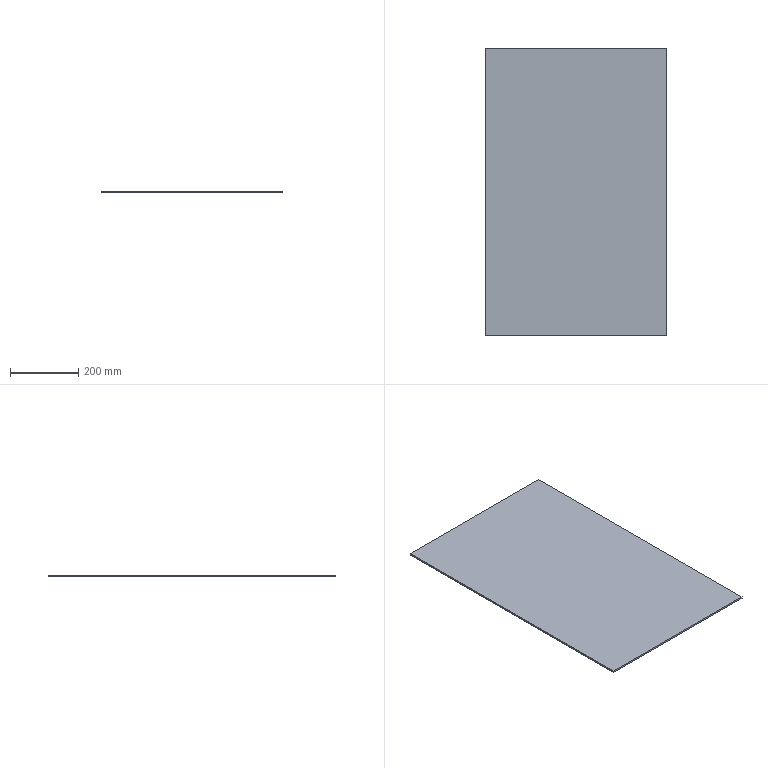Part | SolidWorks | features Extrusion 1, HoleWzd 1 | 1 solid | 6 faces | box 532 x 842 x 5 mm | volume 2239720 mm3 | plane 6
STEP:
#1=CARTESIAN_POINT('',(266.,-421.,0.));
#2=VERTEX_POINT('',#1);
#3=CARTESIAN_POINT('',(266.,421.,0.));
#4=VERTEX_POINT('',#3);
#5=CARTESIAN_POINT('',(266.,421.,0.));
#6=DIRECTION('',(0.,1.,0.));
#7=VECTOR('',#6,1000.);
#8=LINE('',#5,#7);
#9=EDGE_CURVE('',#2,#4,#8,.T.);
#10=ORIENTED_EDGE('',*,*,#9,.T.);
#11=CARTESIAN_POINT('',(266.,421.,5.));
#12=VERTEX_POINT('',#11);
#13=CARTESIAN_POINT('',(266.,421.,5.));
#14=DIRECTION('',(0.,0.,-1.));
#15=VECTOR('',#14,1000.);
#16=LINE('',#13,#15);
#17=EDGE_CURVE('',#12,#4,#16,.T.);
#18=ORIENTED_EDGE('',*,*,#17,.F.);
#19=CARTESIAN_POINT('',(266.,-421.,5.));
#20=VERTEX_POINT('',#19);
#21=CARTESIAN_POINT('',(266.,421.,5.));
#22=DIRECTION('',(0.,1.,0.));
#23=VECTOR('',#22,1000.);
#24=LINE('',#21,#23);
#25=EDGE_CURVE('',#20,#12,#24,.T.);
#26=ORIENTED_EDGE('',*,*,#25,.F.);
#27=CARTESIAN_POINT('',(266.,-421.,5.));
#28=DIRECTION('',(0.,0.,-1.));
#29=VECTOR('',#28,1000.);
#30=LINE('',#27,#29);
#31=EDGE_CURVE('',#20,#2,#30,.T.);
#32=ORIENTED_EDGE('',*,*,#31,.T.);
#33=EDGE_LOOP('',(#10,#18,#26,#32));
#34=FACE_OUTER_BOUND('',#33,.T.);
#35=CARTESIAN_POINT('',(266.,421.,5.));
#36=DIRECTION('',(-1.,0.,0.));
#37=DIRECTION('',(0.,-1.,0.));
#38=AXIS2_PLACEMENT_3D('',#35,#36,#37);
#39=PLANE('',#38);
#40=ADVANCED_FACE('',(#34),#39,.F.);
#41=CARTESIAN_POINT('',(-266.,421.,0.));
#42=VERTEX_POINT('',#41);
#43=CARTESIAN_POINT('',(-266.,421.,0.));
#44=DIRECTION('',(-1.,0.,0.));
#45=VECTOR('',#44,1000.);
#46=LINE('',#43,#45);
#47=EDGE_CURVE('',#4,#42,#46,.T.);
#48=ORIENTED_EDGE('',*,*,#47,.T.);
#49=CARTESIAN_POINT('',(-266.,421.,5.));
#50=VERTEX_POINT('',#49);
#51=CARTESIAN_POINT('',(-266.,421.,5.));
#52=DIRECTION('',(0.,0.,-1.));
#53=VECTOR('',#52,1000.);
#54=LINE('',#51,#53);
#55=EDGE_CURVE('',#50,#42,#54,.T.);
#56=ORIENTED_EDGE('',*,*,#55,.F.);
#57=CARTESIAN_POINT('',(-266.,421.,5.));
#58=DIRECTION('',(-1.,0.,0.));
#59=VECTOR('',#58,1000.);
#60=LINE('',#57,#59);
#61=EDGE_CURVE('',#12,#50,#60,.T.);
#62=ORIENTED_EDGE('',*,*,#61,.F.);
#63=ORIENTED_EDGE('',*,*,#17,.T.);
#64=EDGE_LOOP('',(#48,#56,#62,#63));
#65=FACE_OUTER_BOUND('',#64,.T.);
#66=CARTESIAN_POINT('',(-266.,421.,5.));
#67=DIRECTION('',(0.,-1.,0.));
#68=DIRECTION('',(0.,0.,-1.));
#69=AXIS2_PLACEMENT_3D('',#66,#67,#68);
#70=PLANE('',#69);
#71=ADVANCED_FACE('',(#65),#70,.F.);
#72=CARTESIAN_POINT('',(-266.,-421.,0.));
#73=VERTEX_POINT('',#72);
#74=CARTESIAN_POINT('',(-266.,421.,0.));
#75=DIRECTION('',(0.,-1.,0.));
#76=VECTOR('',#75,1000.);
#77=LINE('',#74,#76);
#78=EDGE_CURVE('',#42,#73,#77,.T.);
#79=ORIENTED_EDGE('',*,*,#78,.T.);
#80=CARTESIAN_POINT('',(-266.,-421.,5.));
#81=VERTEX_POINT('',#80);
#82=CARTESIAN_POINT('',(-266.,-421.,5.));
#83=DIRECTION('',(0.,0.,-1.));
#84=VECTOR('',#83,1000.);
#85=LINE('',#82,#84);
#86=EDGE_CURVE('',#81,#73,#85,.T.);
#87=ORIENTED_EDGE('',*,*,#86,.F.);
#88=CARTESIAN_POINT('',(-266.,421.,5.));
#89=DIRECTION('',(0.,-1.,0.));
#90=VECTOR('',#89,1000.);
#91=LINE('',#88,#90);
#92=EDGE_CURVE('',#50,#81,#91,.T.);
#93=ORIENTED_EDGE('',*,*,#92,.F.);
#94=ORIENTED_EDGE('',*,*,#55,.T.);
#95=EDGE_LOOP('',(#79,#87,#93,#94));
#96=FACE_OUTER_BOUND('',#95,.T.);
#97=CARTESIAN_POINT('',(-266.,421.,5.));
#98=DIRECTION('',(1.,0.,0.));
#99=DIRECTION('',(0.,1.,0.));
#100=AXIS2_PLACEMENT_3D('',#97,#98,#99);
#101=PLANE('',#100);
#102=ADVANCED_FACE('',(#96),#101,.F.);
#103=CARTESIAN_POINT('',(-266.,-421.,0.));
#104=DIRECTION('',(1.,0.,0.));
#105=VECTOR('',#104,1000.);
#106=LINE('',#103,#105);
#107=EDGE_CURVE('',#73,#2,#106,.T.);
#108=ORIENTED_EDGE('',*,*,#107,.T.);
#109=ORIENTED_EDGE('',*,*,#31,.F.);
#110=CARTESIAN_POINT('',(-266.,-421.,5.));
#111=DIRECTION('',(1.,0.,0.));
#112=VECTOR('',#111,1000.);
#113=LINE('',#110,#112);
#114=EDGE_CURVE('',#81,#20,#113,.T.);
#115=ORIENTED_EDGE('',*,*,#114,.F.);
#116=ORIENTED_EDGE('',*,*,#86,.T.);
#117=EDGE_LOOP('',(#108,#109,#115,#116));
#118=FACE_OUTER_BOUND('',#117,.T.);
#119=CARTESIAN_POINT('',(-266.,-421.,5.));
#120=DIRECTION('',(0.,1.,0.));
#121=DIRECTION('',(0.,0.,1.));
#122=AXIS2_PLACEMENT_3D('',#119,#120,#121);
#123=PLANE('',#122);
#124=ADVANCED_FACE('',(#118),#123,.F.);
#125=ORIENTED_EDGE('',*,*,#25,.T.);
#126=ORIENTED_EDGE('',*,*,#61,.T.);
#127=ORIENTED_EDGE('',*,*,#92,.T.);
#128=ORIENTED_EDGE('',*,*,#114,.T.);
#129=EDGE_LOOP('',(#125,#126,#127,#128));
#130=FACE_OUTER_BOUND('',#129,.T.);
#131=CARTESIAN_POINT('',(0.,0.,5.));
#132=DIRECTION('',(0.,0.,1.));
#133=DIRECTION('',(1.,0.,0.));
#134=AXIS2_PLACEMENT_3D('',#131,#132,#133);
#135=PLANE('',#134);
#136=ADVANCED_FACE('',(#130),#135,.T.);
#137=ORIENTED_EDGE('',*,*,#9,.F.);
#138=ORIENTED_EDGE('',*,*,#107,.F.);
#139=ORIENTED_EDGE('',*,*,#78,.F.);
#140=ORIENTED_EDGE('',*,*,#47,.F.);
#141=EDGE_LOOP('',(#137,#138,#139,#140));
#142=FACE_OUTER_BOUND('',#141,.T.);
#143=CARTESIAN_POINT('',(0.,0.,0.));
#144=DIRECTION('',(0.,0.,1.));
#145=DIRECTION('',(1.,0.,0.));
#146=AXIS2_PLACEMENT_3D('',#143,#144,#145);
#147=PLANE('',#146);
#148=ADVANCED_FACE('',(#142),#147,.F.);
#149=CLOSED_SHELL('',(#40,#71,#102,#124,#136,#148));
#150=MANIFOLD_SOLID_BREP('',#149);
#151=CARTESIAN_POINT('',(0.,0.,0.));
#152=DIRECTION('',(0.,0.,1.));
#153=DIRECTION('',(1.,0.,0.));
#154=AXIS2_PLACEMENT_3D('',#151,#152,#153);
#155=(LENGTH_UNIT()NAMED_UNIT(*)SI_UNIT(.MILLI.,.METRE.));
#156=UNCERTAINTY_MEASURE_WITH_UNIT(LENGTH_MEASURE(0.00001),#155,'','');
#157=(NAMED_UNIT(*)PLANE_ANGLE_UNIT()SI_UNIT($,.RADIAN.));
#158=(NAMED_UNIT(*)SI_UNIT($,.STERADIAN.)SOLID_ANGLE_UNIT());
#159=(GEOMETRIC_REPRESENTATION_CONTEXT(3)GLOBAL_UNCERTAINTY_ASSIGNED_CONTEXT((#156))GLOBAL_UNIT_ASSIGNED_CONTEXT((#155,#157,#158))REPRESENTATION_CONTEXT('',''));
#160=ADVANCED_BREP_SHAPE_REPRESENTATION('',(#150,#154),#159);